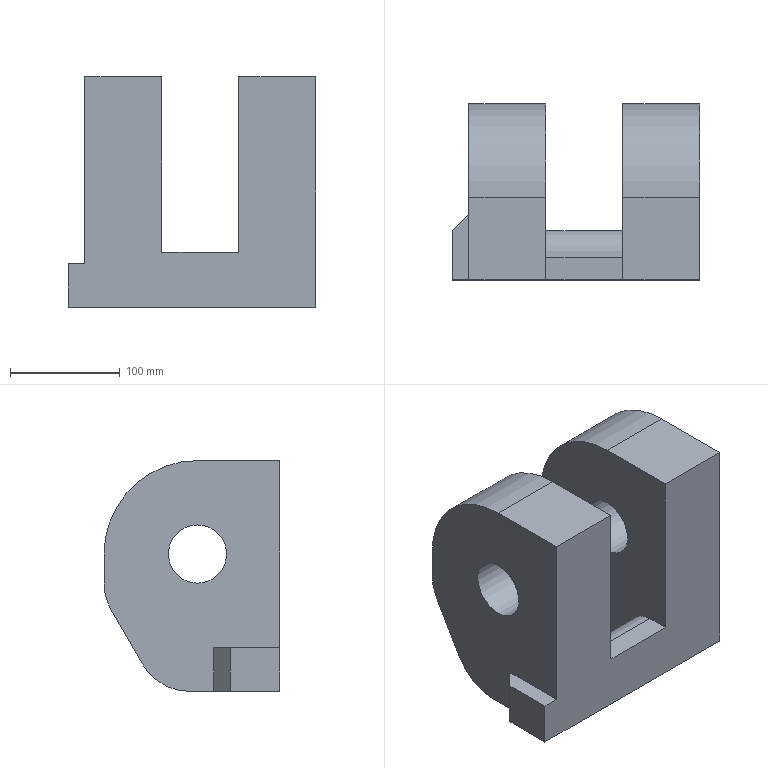Part | NX | features solid 2 | 1 solid | 25 faces | box 225 x 160 x 210 mm | volume 4033518 mm3 | plane 16 | cylinder 9 | commonest cylinder face diameters 100 x4 53 x2 170 x2 50 x1
STEP:
#1=CARTESIAN_POINT('',(-925.,625.,-221.5));
#2=VERTEX_POINT('',#1);
#3=CARTESIAN_POINT('',(-925.,625.,-195.));
#4=DIRECTION('',(1.,0.,0.));
#5=DIRECTION('',(0.,0.,-1.));
#6=AXIS2_PLACEMENT_3D('',#3,#4,#5);
#7=CIRCLE('',#6,26.5);
#8=EDGE_CURVE('',#2,#2,#7,.T.);
#9=ORIENTED_EDGE('',*,*,#8,.T.);
#10=EDGE_LOOP('',(#9));
#11=FACE_BOUND('',#10,.T.);
#12=CARTESIAN_POINT('',(-995.,625.,-221.5));
#13=VERTEX_POINT('',#12);
#14=CARTESIAN_POINT('',(-995.,625.,-195.));
#15=DIRECTION('',(1.,0.,0.));
#16=DIRECTION('',(0.,0.,-1.));
#17=AXIS2_PLACEMENT_3D('',#14,#15,#16);
#18=CIRCLE('',#17,26.5);
#19=EDGE_CURVE('',#13,#13,#18,.T.);
#20=ORIENTED_EDGE('',*,*,#19,.F.);
#21=EDGE_LOOP('',(#20));
#22=FACE_BOUND('',#21,.T.);
#23=CARTESIAN_POINT('',(-915.,625.,-195.));
#24=DIRECTION('',(-1.,0.,0.));
#25=DIRECTION('',(0.,0.,-1.));
#26=AXIS2_PLACEMENT_3D('',#23,#24,#25);
#27=CYLINDRICAL_SURFACE('',#26,26.5);
#28=ADVANCED_FACE('',(#11,#22),#27,.F.);
#29=CARTESIAN_POINT('',(-995.,631.906,-320.));
#30=VERTEX_POINT('',#29);
#31=CARTESIAN_POINT('',(-995.,675.207,-295.));
#32=VERTEX_POINT('',#31);
#33=CARTESIAN_POINT('',(-995.,631.906,-270.));
#34=DIRECTION('',(1.,0.,0.));
#35=DIRECTION('',(0.,0.,-1.));
#36=AXIS2_PLACEMENT_3D('',#33,#34,#35);
#37=CIRCLE('',#36,50.);
#38=EDGE_CURVE('',#30,#32,#37,.T.);
#39=ORIENTED_EDGE('',*,*,#38,.T.);
#40=CARTESIAN_POINT('',(-925.,675.207,-295.));
#41=VERTEX_POINT('',#40);
#42=CARTESIAN_POINT('',(-915.,675.207,-295.));
#43=DIRECTION('',(-1.,0.,0.));
#44=VECTOR('',#43,1000.);
#45=LINE('',#42,#44);
#46=EDGE_CURVE('',#41,#32,#45,.T.);
#47=ORIENTED_EDGE('',*,*,#46,.F.);
#48=CARTESIAN_POINT('',(-925.,631.906,-320.));
#49=VERTEX_POINT('',#48);
#50=CARTESIAN_POINT('',(-925.,631.906,-270.));
#51=DIRECTION('',(1.,0.,0.));
#52=DIRECTION('',(0.,0.,-1.));
#53=AXIS2_PLACEMENT_3D('',#50,#51,#52);
#54=CIRCLE('',#53,50.);
#55=EDGE_CURVE('',#49,#41,#54,.T.);
#56=ORIENTED_EDGE('',*,*,#55,.F.);
#57=CARTESIAN_POINT('',(-915.,631.906,-320.));
#58=DIRECTION('',(-1.,0.,0.));
#59=VECTOR('',#58,1000.);
#60=LINE('',#57,#59);
#61=EDGE_CURVE('',#49,#30,#60,.T.);
#62=ORIENTED_EDGE('',*,*,#61,.T.);
#63=EDGE_LOOP('',(#39,#47,#56,#62));
#64=FACE_BOUND('',#63,.T.);
#65=CARTESIAN_POINT('',(-915.,631.906,-270.));
#66=DIRECTION('',(-1.,0.,0.));
#67=DIRECTION('',(0.,0.,-1.));
#68=AXIS2_PLACEMENT_3D('',#65,#66,#67);
#69=CYLINDRICAL_SURFACE('',#68,50.);
#70=ADVANCED_FACE('',(#64),#69,.T.);
#71=CARTESIAN_POINT('',(-995.,703.301,-246.34));
#72=VERTEX_POINT('',#71);
#73=CARTESIAN_POINT('',(-995.,655.,-330.));
#74=DIRECTION('',(0.,0.5,0.866));
#75=VECTOR('',#74,1000.);
#76=LINE('',#73,#75);
#77=EDGE_CURVE('',#32,#72,#76,.T.);
#78=ORIENTED_EDGE('',*,*,#77,.T.);
#79=CARTESIAN_POINT('',(-925.,703.301,-246.34));
#80=VERTEX_POINT('',#79);
#81=CARTESIAN_POINT('',(-915.,703.301,-246.34));
#82=DIRECTION('',(-1.,0.,0.));
#83=VECTOR('',#82,1000.);
#84=LINE('',#81,#83);
#85=EDGE_CURVE('',#80,#72,#84,.T.);
#86=ORIENTED_EDGE('',*,*,#85,.F.);
#87=CARTESIAN_POINT('',(-925.,655.,-330.));
#88=DIRECTION('',(0.,0.5,0.866));
#89=VECTOR('',#88,1000.);
#90=LINE('',#87,#89);
#91=EDGE_CURVE('',#41,#80,#90,.T.);
#92=ORIENTED_EDGE('',*,*,#91,.F.);
#93=ORIENTED_EDGE('',*,*,#46,.T.);
#94=EDGE_LOOP('',(#78,#86,#92,#93));
#95=FACE_BOUND('',#94,.T.);
#96=CARTESIAN_POINT('',(-915.,655.,-330.));
#97=DIRECTION('',(0.,-0.866,0.5));
#98=DIRECTION('',(0.,0.5,0.866));
#99=AXIS2_PLACEMENT_3D('',#96,#97,#98);
#100=PLANE('',#99);
#101=ADVANCED_FACE('',(#95),#100,.F.);
#102=CARTESIAN_POINT('',(-995.,710.,-221.34));
#103=VERTEX_POINT('',#102);
#104=CARTESIAN_POINT('',(-995.,660.,-221.34));
#105=DIRECTION('',(1.,0.,0.));
#106=DIRECTION('',(0.,0.,-1.));
#107=AXIS2_PLACEMENT_3D('',#104,#105,#106);
#108=CIRCLE('',#107,50.);
#109=EDGE_CURVE('',#72,#103,#108,.T.);
#110=ORIENTED_EDGE('',*,*,#109,.T.);
#111=CARTESIAN_POINT('',(-925.,710.,-221.34));
#112=VERTEX_POINT('',#111);
#113=CARTESIAN_POINT('',(-915.,710.,-221.34));
#114=DIRECTION('',(-1.,0.,0.));
#115=VECTOR('',#114,1000.);
#116=LINE('',#113,#115);
#117=EDGE_CURVE('',#112,#103,#116,.T.);
#118=ORIENTED_EDGE('',*,*,#117,.F.);
#119=CARTESIAN_POINT('',(-925.,660.,-221.34));
#120=DIRECTION('',(1.,0.,0.));
#121=DIRECTION('',(0.,0.,-1.));
#122=AXIS2_PLACEMENT_3D('',#119,#120,#121);
#123=CIRCLE('',#122,50.);
#124=EDGE_CURVE('',#80,#112,#123,.T.);
#125=ORIENTED_EDGE('',*,*,#124,.F.);
#126=ORIENTED_EDGE('',*,*,#85,.T.);
#127=EDGE_LOOP('',(#110,#118,#125,#126));
#128=FACE_BOUND('',#127,.T.);
#129=CARTESIAN_POINT('',(-915.,660.,-221.34));
#130=DIRECTION('',(-1.,0.,0.));
#131=DIRECTION('',(0.,0.,-1.));
#132=AXIS2_PLACEMENT_3D('',#129,#130,#131);
#133=CYLINDRICAL_SURFACE('',#132,50.);
#134=ADVANCED_FACE('',(#128),#133,.T.);
#135=CARTESIAN_POINT('',(-995.,710.,-195.));
#136=VERTEX_POINT('',#135);
#137=CARTESIAN_POINT('',(-995.,710.,-195.));
#138=DIRECTION('',(0.,0.,-1.));
#139=VECTOR('',#138,1000.);
#140=LINE('',#137,#139);
#141=EDGE_CURVE('',#136,#103,#140,.T.);
#142=ORIENTED_EDGE('',*,*,#141,.F.);
#143=CARTESIAN_POINT('',(-925.,710.,-195.));
#144=VERTEX_POINT('',#143);
#145=CARTESIAN_POINT('',(-915.,710.,-195.));
#146=DIRECTION('',(-1.,0.,0.));
#147=VECTOR('',#146,1000.);
#148=LINE('',#145,#147);
#149=EDGE_CURVE('',#144,#136,#148,.T.);
#150=ORIENTED_EDGE('',*,*,#149,.F.);
#151=CARTESIAN_POINT('',(-925.,710.,-195.));
#152=DIRECTION('',(0.,0.,-1.));
#153=VECTOR('',#152,1000.);
#154=LINE('',#151,#153);
#155=EDGE_CURVE('',#144,#112,#154,.T.);
#156=ORIENTED_EDGE('',*,*,#155,.T.);
#157=ORIENTED_EDGE('',*,*,#117,.T.);
#158=EDGE_LOOP('',(#142,#150,#156,#157));
#159=FACE_BOUND('',#158,.T.);
#160=CARTESIAN_POINT('',(-915.,710.,-195.));
#161=DIRECTION('',(0.,1.,0.));
#162=DIRECTION('',(0.,0.,-1.));
#163=AXIS2_PLACEMENT_3D('',#160,#161,#162);
#164=PLANE('',#163);
#165=ADVANCED_FACE('',(#159),#164,.T.);
#166=CARTESIAN_POINT('',(-995.,570.,-270.));
#167=VERTEX_POINT('',#166);
#168=CARTESIAN_POINT('',(-995.,570.,-320.));
#169=VERTEX_POINT('',#168);
#170=CARTESIAN_POINT('',(-995.,570.,-295.));
#171=DIRECTION('',(-1.,0.,0.));
#172=DIRECTION('',(0.,0.,-1.));
#173=AXIS2_PLACEMENT_3D('',#170,#171,#172);
#174=CIRCLE('',#173,25.);
#175=EDGE_CURVE('',#167,#169,#174,.T.);
#176=ORIENTED_EDGE('',*,*,#175,.T.);
#177=CARTESIAN_POINT('',(-1045.001,570.,-320.));
#178=VERTEX_POINT('',#177);
#179=CARTESIAN_POINT('',(-975.001,570.,-320.));
#180=DIRECTION('',(-1.,0.,0.));
#181=VECTOR('',#180,1000.);
#182=LINE('',#179,#181);
#183=EDGE_CURVE('',#178,#169,#182,.F.);
#184=ORIENTED_EDGE('',*,*,#183,.F.);
#185=CARTESIAN_POINT('',(-1065.,570.,-320.));
#186=VERTEX_POINT('',#185);
#187=CARTESIAN_POINT('',(-1055.,570.,-320.));
#188=DIRECTION('',(1.,0.,0.));
#189=VECTOR('',#188,1000.);
#190=LINE('',#187,#189);
#191=EDGE_CURVE('',#186,#178,#190,.T.);
#192=ORIENTED_EDGE('',*,*,#191,.F.);
#193=CARTESIAN_POINT('',(-1065.,570.,-270.));
#194=VERTEX_POINT('',#193);
#195=CARTESIAN_POINT('',(-1065.,570.,-295.));
#196=DIRECTION('',(-1.,0.,0.));
#197=DIRECTION('',(0.,0.,-1.));
#198=AXIS2_PLACEMENT_3D('',#195,#196,#197);
#199=CIRCLE('',#198,25.);
#200=EDGE_CURVE('',#194,#186,#199,.T.);
#201=ORIENTED_EDGE('',*,*,#200,.F.);
#202=CARTESIAN_POINT('',(-975.001,570.,-270.));
#203=DIRECTION('',(-1.,0.,0.));
#204=VECTOR('',#203,1000.);
#205=LINE('',#202,#204);
#206=EDGE_CURVE('',#167,#194,#205,.T.);
#207=ORIENTED_EDGE('',*,*,#206,.F.);
#208=EDGE_LOOP('',(#176,#184,#192,#201,#207));
#209=FACE_BOUND('',#208,.T.);
#210=CARTESIAN_POINT('',(-975.001,570.,-295.));
#211=DIRECTION('',(-1.,0.,0.));
#212=DIRECTION('',(0.,-1.,0.));
#213=AXIS2_PLACEMENT_3D('',#210,#211,#212);
#214=CYLINDRICAL_SURFACE('',#213,25.);
#215=ADVANCED_FACE('',(#209),#214,.T.);
#216=CARTESIAN_POINT('',(-1065.,710.,-195.));
#217=VERTEX_POINT('',#216);
#218=CARTESIAN_POINT('',(-1065.,710.,-221.34));
#219=VERTEX_POINT('',#218);
#220=CARTESIAN_POINT('',(-1065.,710.,-195.));
#221=DIRECTION('',(0.,0.,-1.));
#222=VECTOR('',#221,1000.);
#223=LINE('',#220,#222);
#224=EDGE_CURVE('',#217,#219,#223,.T.);
#225=ORIENTED_EDGE('',*,*,#224,.T.);
#226=CARTESIAN_POINT('',(-1135.,710.,-221.34));
#227=VERTEX_POINT('',#226);
#228=CARTESIAN_POINT('',(-1125.,710.,-221.34));
#229=DIRECTION('',(-1.,0.,0.));
#230=VECTOR('',#229,1000.);
#231=LINE('',#228,#230);
#232=EDGE_CURVE('',#219,#227,#231,.T.);
#233=ORIENTED_EDGE('',*,*,#232,.T.);
#234=CARTESIAN_POINT('',(-1135.,710.,-195.));
#235=VERTEX_POINT('',#234);
#236=CARTESIAN_POINT('',(-1135.,710.,-195.));
#237=DIRECTION('',(0.,0.,-1.));
#238=VECTOR('',#237,1000.);
#239=LINE('',#236,#238);
#240=EDGE_CURVE('',#235,#227,#239,.T.);
#241=ORIENTED_EDGE('',*,*,#240,.F.);
#242=CARTESIAN_POINT('',(-1125.,710.,-195.));
#243=DIRECTION('',(1.,0.,0.));
#244=VECTOR('',#243,1000.);
#245=LINE('',#242,#244);
#246=EDGE_CURVE('',#235,#217,#245,.T.);
#247=ORIENTED_EDGE('',*,*,#246,.T.);
#248=EDGE_LOOP('',(#225,#233,#241,#247));
#249=FACE_BOUND('',#248,.T.);
#250=CARTESIAN_POINT('',(-1125.,710.,-195.));
#251=DIRECTION('',(0.,-1.,0.));
#252=DIRECTION('',(0.,0.,1.));
#253=AXIS2_PLACEMENT_3D('',#250,#251,#252);
#254=PLANE('',#253);
#255=ADVANCED_FACE('',(#249),#254,.F.);
#256=CARTESIAN_POINT('',(-1135.,703.301,-246.34));
#257=VERTEX_POINT('',#256);
#258=CARTESIAN_POINT('',(-1135.,660.,-221.34));
#259=DIRECTION('',(-1.,0.,0.));
#260=DIRECTION('',(0.,1.,0.));
#261=AXIS2_PLACEMENT_3D('',#258,#259,#260);
#262=CIRCLE('',#261,50.);
#263=EDGE_CURVE('',#227,#257,#262,.T.);
#264=ORIENTED_EDGE('',*,*,#263,.F.);
#265=ORIENTED_EDGE('',*,*,#232,.F.);
#266=CARTESIAN_POINT('',(-1065.,703.301,-246.34));
#267=VERTEX_POINT('',#266);
#268=CARTESIAN_POINT('',(-1065.,660.,-221.34));
#269=DIRECTION('',(1.,0.,0.));
#270=DIRECTION('',(0.,0.,-1.));
#271=AXIS2_PLACEMENT_3D('',#268,#269,#270);
#272=CIRCLE('',#271,50.);
#273=EDGE_CURVE('',#267,#219,#272,.T.);
#274=ORIENTED_EDGE('',*,*,#273,.F.);
#275=CARTESIAN_POINT('',(-1055.,703.301,-246.34));
#276=DIRECTION('',(1.,0.,0.));
#277=VECTOR('',#276,1000.);
#278=LINE('',#275,#277);
#279=EDGE_CURVE('',#257,#267,#278,.T.);
#280=ORIENTED_EDGE('',*,*,#279,.F.);
#281=EDGE_LOOP('',(#264,#265,#274,#280));
#282=FACE_BOUND('',#281,.T.);
#283=CARTESIAN_POINT('',(-1125.,660.,-221.34));
#284=DIRECTION('',(-1.,0.,0.));
#285=DIRECTION('',(0.,0.,-1.));
#286=AXIS2_PLACEMENT_3D('',#283,#284,#285);
#287=CYLINDRICAL_SURFACE('',#286,50.);
#288=ADVANCED_FACE('',(#282),#287,.T.);
#289=CARTESIAN_POINT('',(-1065.,675.207,-295.));
#290=VERTEX_POINT('',#289);
#291=CARTESIAN_POINT('',(-1065.,655.,-330.));
#292=DIRECTION('',(0.,0.5,0.866));
#293=VECTOR('',#292,1000.);
#294=LINE('',#291,#293);
#295=EDGE_CURVE('',#290,#267,#294,.T.);
#296=ORIENTED_EDGE('',*,*,#295,.F.);
#297=CARTESIAN_POINT('',(-1135.,675.207,-295.));
#298=VERTEX_POINT('',#297);
#299=CARTESIAN_POINT('',(-1125.,675.207,-295.));
#300=DIRECTION('',(-1.,0.,0.));
#301=VECTOR('',#300,1000.);
#302=LINE('',#299,#301);
#303=EDGE_CURVE('',#290,#298,#302,.T.);
#304=ORIENTED_EDGE('',*,*,#303,.T.);
#305=CARTESIAN_POINT('',(-1135.,655.,-330.));
#306=DIRECTION('',(0.,0.5,0.866));
#307=VECTOR('',#306,1000.);
#308=LINE('',#305,#307);
#309=EDGE_CURVE('',#298,#257,#308,.T.);
#310=ORIENTED_EDGE('',*,*,#309,.T.);
#311=ORIENTED_EDGE('',*,*,#279,.T.);
#312=EDGE_LOOP('',(#296,#304,#310,#311));
#313=FACE_BOUND('',#312,.T.);
#314=CARTESIAN_POINT('',(-1125.,655.,-330.));
#315=DIRECTION('',(0.,0.866,-0.5));
#316=DIRECTION('',(0.,-0.5,-0.866));
#317=AXIS2_PLACEMENT_3D('',#314,#315,#316);
#318=PLANE('',#317);
#319=ADVANCED_FACE('',(#313),#318,.T.);
#320=CARTESIAN_POINT('',(-1135.,631.906,-320.));
#321=VERTEX_POINT('',#320);
#322=CARTESIAN_POINT('',(-1135.,631.906,-270.));
#323=DIRECTION('',(-1.,0.,0.));
#324=DIRECTION('',(0.,1.,0.));
#325=AXIS2_PLACEMENT_3D('',#322,#323,#324);
#326=CIRCLE('',#325,50.);
#327=EDGE_CURVE('',#298,#321,#326,.T.);
#328=ORIENTED_EDGE('',*,*,#327,.F.);
#329=ORIENTED_EDGE('',*,*,#303,.F.);
#330=CARTESIAN_POINT('',(-1065.,631.906,-320.));
#331=VERTEX_POINT('',#330);
#332=CARTESIAN_POINT('',(-1065.,631.906,-270.));
#333=DIRECTION('',(1.,0.,0.));
#334=DIRECTION('',(0.,0.,-1.));
#335=AXIS2_PLACEMENT_3D('',#332,#333,#334);
#336=CIRCLE('',#335,50.);
#337=EDGE_CURVE('',#331,#290,#336,.T.);
#338=ORIENTED_EDGE('',*,*,#337,.F.);
#339=CARTESIAN_POINT('',(-1145.001,631.906,-320.));
#340=DIRECTION('',(1.,0.,0.));
#341=VECTOR('',#340,1000.);
#342=LINE('',#339,#341);
#343=EDGE_CURVE('',#321,#331,#342,.T.);
#344=ORIENTED_EDGE('',*,*,#343,.F.);
#345=EDGE_LOOP('',(#328,#329,#338,#344));
#346=FACE_BOUND('',#345,.T.);
#347=CARTESIAN_POINT('',(-1145.001,631.906,-270.));
#348=DIRECTION('',(1.,0.,0.));
#349=DIRECTION('',(0.,0.,1.));
#350=AXIS2_PLACEMENT_3D('',#347,#348,#349);
#351=CYLINDRICAL_SURFACE('',#350,50.);
#352=ADVANCED_FACE('',(#346),#351,.T.);
#353=CARTESIAN_POINT('',(-1135.,625.,-168.5));
#354=VERTEX_POINT('',#353);
#355=CARTESIAN_POINT('',(-1135.,625.,-195.));
#356=DIRECTION('',(1.,0.,0.));
#357=DIRECTION('',(0.,0.,1.));
#358=AXIS2_PLACEMENT_3D('',#355,#356,#357);
#359=CIRCLE('',#358,26.5);
#360=EDGE_CURVE('',#354,#354,#359,.T.);
#361=ORIENTED_EDGE('',*,*,#360,.F.);
#362=EDGE_LOOP('',(#361));
#363=FACE_BOUND('',#362,.T.);
#364=CARTESIAN_POINT('',(-1065.,625.,-221.5));
#365=VERTEX_POINT('',#364);
#366=CARTESIAN_POINT('',(-1065.,625.,-195.));
#367=DIRECTION('',(1.,0.,0.));
#368=DIRECTION('',(0.,0.,-1.));
#369=AXIS2_PLACEMENT_3D('',#366,#367,#368);
#370=CIRCLE('',#369,26.5);
#371=EDGE_CURVE('',#365,#365,#370,.T.);
#372=ORIENTED_EDGE('',*,*,#371,.T.);
#373=EDGE_LOOP('',(#372));
#374=FACE_BOUND('',#373,.T.);
#375=CARTESIAN_POINT('',(-905.001,625.,-195.));
#376=DIRECTION('',(-1.,0.,0.));
#377=DIRECTION('',(0.,-1.,0.));
#378=AXIS2_PLACEMENT_3D('',#375,#376,#377);
#379=CYLINDRICAL_SURFACE('',#378,26.5);
#380=ADVANCED_FACE('',(#363,#374),#379,.F.);
#381=CARTESIAN_POINT('',(-995.,625.,-110.));
#382=VERTEX_POINT('',#381);
#383=CARTESIAN_POINT('',(-995.,625.,-195.));
#384=DIRECTION('',(-1.,0.,0.));
#385=DIRECTION('',(0.,0.,-1.));
#386=AXIS2_PLACEMENT_3D('',#383,#384,#385);
#387=CIRCLE('',#386,85.);
#388=EDGE_CURVE('',#382,#136,#387,.T.);
#389=ORIENTED_EDGE('',*,*,#388,.F.);
#390=CARTESIAN_POINT('',(-925.,625.,-110.));
#391=VERTEX_POINT('',#390);
#392=CARTESIAN_POINT('',(-915.,625.,-110.));
#393=DIRECTION('',(-1.,0.,0.));
#394=VECTOR('',#393,1000.);
#395=LINE('',#392,#394);
#396=EDGE_CURVE('',#391,#382,#395,.T.);
#397=ORIENTED_EDGE('',*,*,#396,.F.);
#398=CARTESIAN_POINT('',(-925.,625.,-195.));
#399=DIRECTION('',(-1.,0.,0.));
#400=DIRECTION('',(0.,0.,-1.));
#401=AXIS2_PLACEMENT_3D('',#398,#399,#400);
#402=CIRCLE('',#401,85.);
#403=EDGE_CURVE('',#391,#144,#402,.T.);
#404=ORIENTED_EDGE('',*,*,#403,.T.);
#405=ORIENTED_EDGE('',*,*,#149,.T.);
#406=EDGE_LOOP('',(#389,#397,#404,#405));
#407=FACE_BOUND('',#406,.T.);
#408=CARTESIAN_POINT('',(-915.,625.,-195.));
#409=DIRECTION('',(-1.,0.,0.));
#410=DIRECTION('',(0.,0.,-1.));
#411=AXIS2_PLACEMENT_3D('',#408,#409,#410);
#412=CYLINDRICAL_SURFACE('',#411,85.);
#413=ADVANCED_FACE('',(#407),#412,.T.);
#414=CARTESIAN_POINT('',(-1065.,625.,-110.));
#415=VERTEX_POINT('',#414);
#416=CARTESIAN_POINT('',(-1065.,625.,-195.));
#417=DIRECTION('',(-1.,0.,0.));
#418=DIRECTION('',(0.,0.,-1.));
#419=AXIS2_PLACEMENT_3D('',#416,#417,#418);
#420=CIRCLE('',#419,85.);
#421=EDGE_CURVE('',#415,#217,#420,.T.);
#422=ORIENTED_EDGE('',*,*,#421,.T.);
#423=ORIENTED_EDGE('',*,*,#246,.F.);
#424=CARTESIAN_POINT('',(-1135.,625.,-110.));
#425=VERTEX_POINT('',#424);
#426=CARTESIAN_POINT('',(-1135.,625.,-195.));
#427=DIRECTION('',(-1.,0.,0.));
#428=DIRECTION('',(0.,0.,1.));
#429=AXIS2_PLACEMENT_3D('',#426,#427,#428);
#430=CIRCLE('',#429,85.);
#431=EDGE_CURVE('',#425,#235,#430,.T.);
#432=ORIENTED_EDGE('',*,*,#431,.F.);
#433=CARTESIAN_POINT('',(-1045.001,625.,-110.));
#434=DIRECTION('',(-1.,0.,0.));
#435=VECTOR('',#434,1000.);
#436=LINE('',#433,#435);
#437=EDGE_CURVE('',#415,#425,#436,.T.);
#438=ORIENTED_EDGE('',*,*,#437,.F.);
#439=EDGE_LOOP('',(#422,#423,#432,#438));
#440=FACE_BOUND('',#439,.T.);
#441=CARTESIAN_POINT('',(-1045.001,625.,-195.));
#442=DIRECTION('',(-1.,0.,0.));
#443=DIRECTION('',(0.,-1.,0.));
#444=AXIS2_PLACEMENT_3D('',#441,#442,#443);
#445=CYLINDRICAL_SURFACE('',#444,85.);
#446=ADVANCED_FACE('',(#440),#445,.T.);
#447=CARTESIAN_POINT('',(-995.,550.,-270.));
#448=VERTEX_POINT('',#447);
#449=CARTESIAN_POINT('',(-995.,710.,-270.));
#450=DIRECTION('',(0.,1.,0.));
#451=VECTOR('',#450,1000.);
#452=LINE('',#449,#451);
#453=EDGE_CURVE('',#448,#167,#452,.T.);
#454=ORIENTED_EDGE('',*,*,#453,.T.);
#455=ORIENTED_EDGE('',*,*,#206,.T.);
#456=CARTESIAN_POINT('',(-1065.,550.,-270.));
#457=VERTEX_POINT('',#456);
#458=CARTESIAN_POINT('',(-1065.,710.,-270.));
#459=DIRECTION('',(0.,1.,0.));
#460=VECTOR('',#459,1000.);
#461=LINE('',#458,#460);
#462=EDGE_CURVE('',#457,#194,#461,.T.);
#463=ORIENTED_EDGE('',*,*,#462,.F.);
#464=CARTESIAN_POINT('',(-975.001,550.,-270.));
#465=DIRECTION('',(-1.,0.,0.));
#466=VECTOR('',#465,1000.);
#467=LINE('',#464,#466);
#468=EDGE_CURVE('',#448,#457,#467,.T.);
#469=ORIENTED_EDGE('',*,*,#468,.F.);
#470=EDGE_LOOP('',(#454,#455,#463,#469));
#471=FACE_BOUND('',#470,.T.);
#472=CARTESIAN_POINT('',(-975.001,550.,-270.));
#473=DIRECTION('',(0.,0.,-1.));
#474=DIRECTION('',(0.,1.,0.));
#475=AXIS2_PLACEMENT_3D('',#472,#473,#474);
#476=PLANE('',#475);
#477=ADVANCED_FACE('',(#471),#476,.F.);
#478=CARTESIAN_POINT('',(-1065.,550.,-110.));
#479=VERTEX_POINT('',#478);
#480=CARTESIAN_POINT('',(-1065.,710.,-110.));
#481=DIRECTION('',(0.,1.,0.));
#482=VECTOR('',#481,1000.);
#483=LINE('',#480,#482);
#484=EDGE_CURVE('',#479,#415,#483,.T.);
#485=ORIENTED_EDGE('',*,*,#484,.T.);
#486=ORIENTED_EDGE('',*,*,#437,.T.);
#487=CARTESIAN_POINT('',(-1135.,550.,-110.));
#488=VERTEX_POINT('',#487);
#489=CARTESIAN_POINT('',(-1135.,70.,-110.));
#490=DIRECTION('',(0.,1.,0.));
#491=VECTOR('',#490,1000.);
#492=LINE('',#489,#491);
#493=EDGE_CURVE('',#488,#425,#492,.T.);
#494=ORIENTED_EDGE('',*,*,#493,.F.);
#495=CARTESIAN_POINT('',(-401.001,550.,-110.));
#496=DIRECTION('',(-1.,0.,0.));
#497=VECTOR('',#496,1000.);
#498=LINE('',#495,#497);
#499=EDGE_CURVE('',#479,#488,#498,.T.);
#500=ORIENTED_EDGE('',*,*,#499,.F.);
#501=EDGE_LOOP('',(#485,#486,#494,#500));
#502=FACE_BOUND('',#501,.T.);
#503=CARTESIAN_POINT('',(-401.001,70.,-110.));
#504=DIRECTION('',(0.,0.,-1.));
#505=DIRECTION('',(-1.,0.,0.));
#506=AXIS2_PLACEMENT_3D('',#503,#504,#505);
#507=PLANE('',#506);
#508=ADVANCED_FACE('',(#502),#507,.F.);
#509=ORIENTED_EDGE('',*,*,#360,.T.);
#510=EDGE_LOOP('',(#509));
#511=FACE_BOUND('',#510,.T.);
#512=CARTESIAN_POINT('',(-1135.,550.,-280.));
#513=VERTEX_POINT('',#512);
#514=CARTESIAN_POINT('',(-1135.,550.,-130.));
#515=DIRECTION('',(0.,0.,-1.));
#516=VECTOR('',#515,1000.);
#517=LINE('',#514,#516);
#518=EDGE_CURVE('',#488,#513,#517,.T.);
#519=ORIENTED_EDGE('',*,*,#518,.F.);
#520=ORIENTED_EDGE('',*,*,#493,.T.);
#521=ORIENTED_EDGE('',*,*,#431,.T.);
#522=ORIENTED_EDGE('',*,*,#240,.T.);
#523=ORIENTED_EDGE('',*,*,#263,.T.);
#524=ORIENTED_EDGE('',*,*,#309,.F.);
#525=ORIENTED_EDGE('',*,*,#327,.T.);
#526=CARTESIAN_POINT('',(-1135.,610.,-320.));
#527=VERTEX_POINT('',#526);
#528=CARTESIAN_POINT('',(-1135.,371.797,-320.));
#529=DIRECTION('',(0.,-1.,0.));
#530=VECTOR('',#529,1000.);
#531=LINE('',#528,#530);
#532=EDGE_CURVE('',#321,#527,#531,.T.);
#533=ORIENTED_EDGE('',*,*,#532,.T.);
#534=CARTESIAN_POINT('',(-1135.,610.,-280.));
#535=VERTEX_POINT('',#534);
#536=CARTESIAN_POINT('',(-1135.,610.,-310.));
#537=DIRECTION('',(0.,0.,1.));
#538=VECTOR('',#537,1000.);
#539=LINE('',#536,#538);
#540=EDGE_CURVE('',#527,#535,#539,.T.);
#541=ORIENTED_EDGE('',*,*,#540,.T.);
#542=CARTESIAN_POINT('',(-1135.,580.,-280.));
#543=DIRECTION('',(0.,1.,0.));
#544=VECTOR('',#543,1000.);
#545=LINE('',#542,#544);
#546=EDGE_CURVE('',#513,#535,#545,.T.);
#547=ORIENTED_EDGE('',*,*,#546,.F.);
#548=EDGE_LOOP('',(#519,#520,#521,#522,#523,#524,#525,#533,#541,#547));
#549=FACE_BOUND('',#548,.T.);
#550=CARTESIAN_POINT('',(-1135.,371.797,-130.));
#551=DIRECTION('',(1.,0.,0.));
#552=DIRECTION('',(0.,0.,1.));
#553=AXIS2_PLACEMENT_3D('',#550,#551,#552);
#554=PLANE('',#553);
#555=ADVANCED_FACE('',(#511,#549),#554,.F.);
#556=ORIENTED_EDGE('',*,*,#371,.F.);
#557=EDGE_LOOP('',(#556));
#558=FACE_BOUND('',#557,.T.);
#559=CARTESIAN_POINT('',(-1065.,550.,-310.));
#560=DIRECTION('',(0.,0.,-1.));
#561=VECTOR('',#560,1000.);
#562=LINE('',#559,#561);
#563=EDGE_CURVE('',#479,#457,#562,.T.);
#564=ORIENTED_EDGE('',*,*,#563,.T.);
#565=ORIENTED_EDGE('',*,*,#462,.T.);
#566=ORIENTED_EDGE('',*,*,#200,.T.);
#567=CARTESIAN_POINT('',(-1065.,-240.,-320.));
#568=DIRECTION('',(0.,-1.,0.));
#569=VECTOR('',#568,1000.);
#570=LINE('',#567,#569);
#571=EDGE_CURVE('',#331,#186,#570,.T.);
#572=ORIENTED_EDGE('',*,*,#571,.F.);
#573=ORIENTED_EDGE('',*,*,#337,.T.);
#574=ORIENTED_EDGE('',*,*,#295,.T.);
#575=ORIENTED_EDGE('',*,*,#273,.T.);
#576=ORIENTED_EDGE('',*,*,#224,.F.);
#577=ORIENTED_EDGE('',*,*,#421,.F.);
#578=ORIENTED_EDGE('',*,*,#484,.F.);
#579=EDGE_LOOP('',(#564,#565,#566,#572,#573,#574,#575,#576,#577,#578));
#580=FACE_BOUND('',#579,.T.);
#581=CARTESIAN_POINT('',(-1065.,710.,-310.));
#582=DIRECTION('',(1.,0.,0.));
#583=DIRECTION('',(0.,0.,1.));
#584=AXIS2_PLACEMENT_3D('',#581,#582,#583);
#585=PLANE('',#584);
#586=ADVANCED_FACE('',(#558,#580),#585,.T.);
#587=CARTESIAN_POINT('',(-925.,550.,-110.));
#588=VERTEX_POINT('',#587);
#589=CARTESIAN_POINT('',(-925.,710.,-110.));
#590=DIRECTION('',(0.,1.,0.));
#591=VECTOR('',#590,1000.);
#592=LINE('',#589,#591);
#593=EDGE_CURVE('',#588,#391,#592,.T.);
#594=ORIENTED_EDGE('',*,*,#593,.T.);
#595=ORIENTED_EDGE('',*,*,#396,.T.);
#596=CARTESIAN_POINT('',(-995.,550.,-110.));
#597=VERTEX_POINT('',#596);
#598=CARTESIAN_POINT('',(-995.,710.,-110.));
#599=DIRECTION('',(0.,1.,0.));
#600=VECTOR('',#599,1000.);
#601=LINE('',#598,#600);
#602=EDGE_CURVE('',#597,#382,#601,.T.);
#603=ORIENTED_EDGE('',*,*,#602,.F.);
#604=CARTESIAN_POINT('',(-401.001,550.,-110.));
#605=DIRECTION('',(-1.,0.,0.));
#606=VECTOR('',#605,1000.);
#607=LINE('',#604,#606);
#608=EDGE_CURVE('',#588,#597,#607,.T.);
#609=ORIENTED_EDGE('',*,*,#608,.F.);
#610=EDGE_LOOP('',(#594,#595,#603,#609));
#611=FACE_BOUND('',#610,.T.);
#612=CARTESIAN_POINT('',(-401.001,70.,-110.));
#613=DIRECTION('',(0.,0.,-1.));
#614=DIRECTION('',(-1.,0.,0.));
#615=AXIS2_PLACEMENT_3D('',#612,#613,#614);
#616=PLANE('',#615);
#617=ADVANCED_FACE('',(#611),#616,.F.);
#618=CARTESIAN_POINT('',(-925.,550.,-320.));
#619=VERTEX_POINT('',#618);
#620=CARTESIAN_POINT('',(-925.,115.,-320.));
#621=DIRECTION('',(0.,1.,0.));
#622=VECTOR('',#621,1000.);
#623=LINE('',#620,#622);
#624=EDGE_CURVE('',#619,#49,#623,.T.);
#625=ORIENTED_EDGE('',*,*,#624,.T.);
#626=ORIENTED_EDGE('',*,*,#55,.T.);
#627=ORIENTED_EDGE('',*,*,#91,.T.);
#628=ORIENTED_EDGE('',*,*,#124,.T.);
#629=ORIENTED_EDGE('',*,*,#155,.F.);
#630=ORIENTED_EDGE('',*,*,#403,.F.);
#631=ORIENTED_EDGE('',*,*,#593,.F.);
#632=CARTESIAN_POINT('',(-925.,550.,-120.));
#633=DIRECTION('',(0.,0.,1.));
#634=VECTOR('',#633,1000.);
#635=LINE('',#632,#634);
#636=EDGE_CURVE('',#619,#588,#635,.T.);
#637=ORIENTED_EDGE('',*,*,#636,.F.);
#638=EDGE_LOOP('',(#625,#626,#627,#628,#629,#630,#631,#637));
#639=FACE_BOUND('',#638,.T.);
#640=ORIENTED_EDGE('',*,*,#8,.F.);
#641=EDGE_LOOP('',(#640));
#642=FACE_BOUND('',#641,.T.);
#643=CARTESIAN_POINT('',(-925.,-305.,-120.));
#644=DIRECTION('',(-1.,0.,0.));
#645=DIRECTION('',(0.,0.,1.));
#646=AXIS2_PLACEMENT_3D('',#643,#644,#645);
#647=PLANE('',#646);
#648=ADVANCED_FACE('',(#639,#642),#647,.F.);
#649=ORIENTED_EDGE('',*,*,#19,.T.);
#650=EDGE_LOOP('',(#649));
#651=FACE_BOUND('',#650,.T.);
#652=ORIENTED_EDGE('',*,*,#602,.T.);
#653=ORIENTED_EDGE('',*,*,#388,.T.);
#654=ORIENTED_EDGE('',*,*,#141,.T.);
#655=ORIENTED_EDGE('',*,*,#109,.F.);
#656=ORIENTED_EDGE('',*,*,#77,.F.);
#657=ORIENTED_EDGE('',*,*,#38,.F.);
#658=CARTESIAN_POINT('',(-995.,-240.,-320.));
#659=DIRECTION('',(0.,-1.,0.));
#660=VECTOR('',#659,1000.);
#661=LINE('',#658,#660);
#662=EDGE_CURVE('',#30,#169,#661,.T.);
#663=ORIENTED_EDGE('',*,*,#662,.T.);
#664=ORIENTED_EDGE('',*,*,#175,.F.);
#665=ORIENTED_EDGE('',*,*,#453,.F.);
#666=CARTESIAN_POINT('',(-995.,550.,-310.));
#667=DIRECTION('',(0.,0.,-1.));
#668=VECTOR('',#667,1000.);
#669=LINE('',#666,#668);
#670=EDGE_CURVE('',#597,#448,#669,.T.);
#671=ORIENTED_EDGE('',*,*,#670,.F.);
#672=EDGE_LOOP('',(#652,#653,#654,#655,#656,#657,#663,#664,#665,#671));
#673=FACE_BOUND('',#672,.T.);
#674=CARTESIAN_POINT('',(-995.,710.,-310.));
#675=DIRECTION('',(1.,0.,0.));
#676=DIRECTION('',(0.,0.,1.));
#677=AXIS2_PLACEMENT_3D('',#674,#675,#676);
#678=PLANE('',#677);
#679=ADVANCED_FACE('',(#651,#673),#678,.F.);
#680=ORIENTED_EDGE('',*,*,#624,.F.);
#681=CARTESIAN_POINT('',(-1150.,550.,-320.));
#682=VERTEX_POINT('',#681);
#683=CARTESIAN_POINT('',(855.,550.,-320.));
#684=DIRECTION('',(1.,0.,0.));
#685=VECTOR('',#684,1000.);
#686=LINE('',#683,#685);
#687=EDGE_CURVE('',#682,#619,#686,.T.);
#688=ORIENTED_EDGE('',*,*,#687,.F.);
#689=CARTESIAN_POINT('',(-1150.,595.,-320.));
#690=VERTEX_POINT('',#689);
#691=CARTESIAN_POINT('',(-1150.,580.,-320.));
#692=DIRECTION('',(0.,1.,0.));
#693=VECTOR('',#692,1000.);
#694=LINE('',#691,#693);
#695=EDGE_CURVE('',#682,#690,#694,.T.);
#696=ORIENTED_EDGE('',*,*,#695,.T.);
#697=CARTESIAN_POINT('',(-1153.75,591.25,-320.));
#698=DIRECTION('',(-0.7071,-0.7071,0.));
#699=VECTOR('',#698,1000.);
#700=LINE('',#697,#699);
#701=EDGE_CURVE('',#527,#690,#700,.T.);
#702=ORIENTED_EDGE('',*,*,#701,.F.);
#703=ORIENTED_EDGE('',*,*,#532,.F.);
#704=ORIENTED_EDGE('',*,*,#343,.T.);
#705=ORIENTED_EDGE('',*,*,#571,.T.);
#706=ORIENTED_EDGE('',*,*,#191,.T.);
#707=ORIENTED_EDGE('',*,*,#183,.T.);
#708=ORIENTED_EDGE('',*,*,#662,.F.);
#709=ORIENTED_EDGE('',*,*,#61,.F.);
#710=EDGE_LOOP('',(#680,#688,#696,#702,#703,#704,#705,#706,#707,#708,#709));
#711=FACE_BOUND('',#710,.T.);
#712=CARTESIAN_POINT('',(855.,115.,-320.));
#713=DIRECTION('',(0.,0.,1.));
#714=DIRECTION('',(0.,-1.,0.));
#715=AXIS2_PLACEMENT_3D('',#712,#713,#714);
#716=PLANE('',#715);
#717=ADVANCED_FACE('',(#711),#716,.F.);
#718=ORIENTED_EDGE('',*,*,#636,.T.);
#719=ORIENTED_EDGE('',*,*,#608,.T.);
#720=ORIENTED_EDGE('',*,*,#670,.T.);
#721=ORIENTED_EDGE('',*,*,#468,.T.);
#722=ORIENTED_EDGE('',*,*,#563,.F.);
#723=ORIENTED_EDGE('',*,*,#499,.T.);
#724=ORIENTED_EDGE('',*,*,#518,.T.);
#725=CARTESIAN_POINT('',(-1150.,550.,-280.));
#726=VERTEX_POINT('',#725);
#727=CARTESIAN_POINT('',(-1142.5,550.,-280.));
#728=DIRECTION('',(1.,0.,0.));
#729=VECTOR('',#728,1000.);
#730=LINE('',#727,#729);
#731=EDGE_CURVE('',#726,#513,#730,.T.);
#732=ORIENTED_EDGE('',*,*,#731,.F.);
#733=CARTESIAN_POINT('',(-1150.,550.,-310.));
#734=DIRECTION('',(0.,0.,1.));
#735=VECTOR('',#734,1000.);
#736=LINE('',#733,#735);
#737=EDGE_CURVE('',#682,#726,#736,.T.);
#738=ORIENTED_EDGE('',*,*,#737,.F.);
#739=ORIENTED_EDGE('',*,*,#687,.T.);
#740=EDGE_LOOP('',(#718,#719,#720,#721,#722,#723,#724,#732,#738,#739));
#741=FACE_BOUND('',#740,.T.);
#742=CARTESIAN_POINT('',(970.,550.,-80.));
#743=DIRECTION('',(0.,1.,0.));
#744=DIRECTION('',(0.,0.,1.));
#745=AXIS2_PLACEMENT_3D('',#742,#743,#744);
#746=PLANE('',#745);
#747=ADVANCED_FACE('',(#741),#746,.F.);
#748=CARTESIAN_POINT('',(-1150.,595.,-280.));
#749=VERTEX_POINT('',#748);
#750=CARTESIAN_POINT('',(-1150.,580.,-280.));
#751=DIRECTION('',(0.,-1.,0.));
#752=VECTOR('',#751,1000.);
#753=LINE('',#750,#752);
#754=EDGE_CURVE('',#749,#726,#753,.T.);
#755=ORIENTED_EDGE('',*,*,#754,.T.);
#756=ORIENTED_EDGE('',*,*,#731,.T.);
#757=ORIENTED_EDGE('',*,*,#546,.T.);
#758=CARTESIAN_POINT('',(-1153.75,591.25,-280.));
#759=DIRECTION('',(0.7071,0.7071,0.));
#760=VECTOR('',#759,1000.);
#761=LINE('',#758,#760);
#762=EDGE_CURVE('',#749,#535,#761,.T.);
#763=ORIENTED_EDGE('',*,*,#762,.F.);
#764=EDGE_LOOP('',(#755,#756,#757,#763));
#765=FACE_BOUND('',#764,.T.);
#766=CARTESIAN_POINT('',(-1142.5,580.,-280.));
#767=DIRECTION('',(0.,0.,1.));
#768=DIRECTION('',(-1.,0.,0.));
#769=AXIS2_PLACEMENT_3D('',#766,#767,#768);
#770=PLANE('',#769);
#771=ADVANCED_FACE('',(#765),#770,.T.);
#772=ORIENTED_EDGE('',*,*,#695,.F.);
#773=ORIENTED_EDGE('',*,*,#737,.T.);
#774=ORIENTED_EDGE('',*,*,#754,.F.);
#775=CARTESIAN_POINT('',(-1150.,595.,-310.));
#776=DIRECTION('',(0.,0.,1.));
#777=VECTOR('',#776,1000.);
#778=LINE('',#775,#777);
#779=EDGE_CURVE('',#690,#749,#778,.T.);
#780=ORIENTED_EDGE('',*,*,#779,.F.);
#781=EDGE_LOOP('',(#772,#773,#774,#780));
#782=FACE_BOUND('',#781,.T.);
#783=CARTESIAN_POINT('',(-1150.,580.,-310.));
#784=DIRECTION('',(-1.,0.,0.));
#785=DIRECTION('',(0.,0.,-1.));
#786=AXIS2_PLACEMENT_3D('',#783,#784,#785);
#787=PLANE('',#786);
#788=ADVANCED_FACE('',(#782),#787,.T.);
#789=ORIENTED_EDGE('',*,*,#701,.T.);
#790=ORIENTED_EDGE('',*,*,#779,.T.);
#791=ORIENTED_EDGE('',*,*,#762,.T.);
#792=ORIENTED_EDGE('',*,*,#540,.F.);
#793=EDGE_LOOP('',(#789,#790,#791,#792));
#794=FACE_BOUND('',#793,.T.);
#795=CARTESIAN_POINT('',(-1150.,595.,-310.));
#796=DIRECTION('',(0.7071,-0.7071,0.));
#797=DIRECTION('',(0.7071,0.7071,0.));
#798=AXIS2_PLACEMENT_3D('',#795,#796,#797);
#799=PLANE('',#798);
#800=ADVANCED_FACE('',(#794),#799,.F.);
#801=CLOSED_SHELL('',(#28,#70,#101,#134,#165,#215,#255,#288,#319,#352,#380,#413,#446,#477,#508,#555,#586,#617,#648,#679,#717,#747,#771,#788,#800));
#802=MANIFOLD_SOLID_BREP('',#801);
#803=(LENGTH_UNIT()NAMED_UNIT(*)SI_UNIT(.MILLI.,.METRE.));
#804=UNCERTAINTY_MEASURE_WITH_UNIT(LENGTH_MEASURE(0.00001),#803,'','');
#805=(NAMED_UNIT(*)PLANE_ANGLE_UNIT()SI_UNIT($,.RADIAN.));
#806=(NAMED_UNIT(*)SI_UNIT($,.STERADIAN.)SOLID_ANGLE_UNIT());
#807=(GEOMETRIC_REPRESENTATION_CONTEXT(3)GLOBAL_UNCERTAINTY_ASSIGNED_CONTEXT((#804))GLOBAL_UNIT_ASSIGNED_CONTEXT((#803,#805,#806))REPRESENTATION_CONTEXT('',''));
#808=ADVANCED_BREP_SHAPE_REPRESENTATION('',(#802),#807);